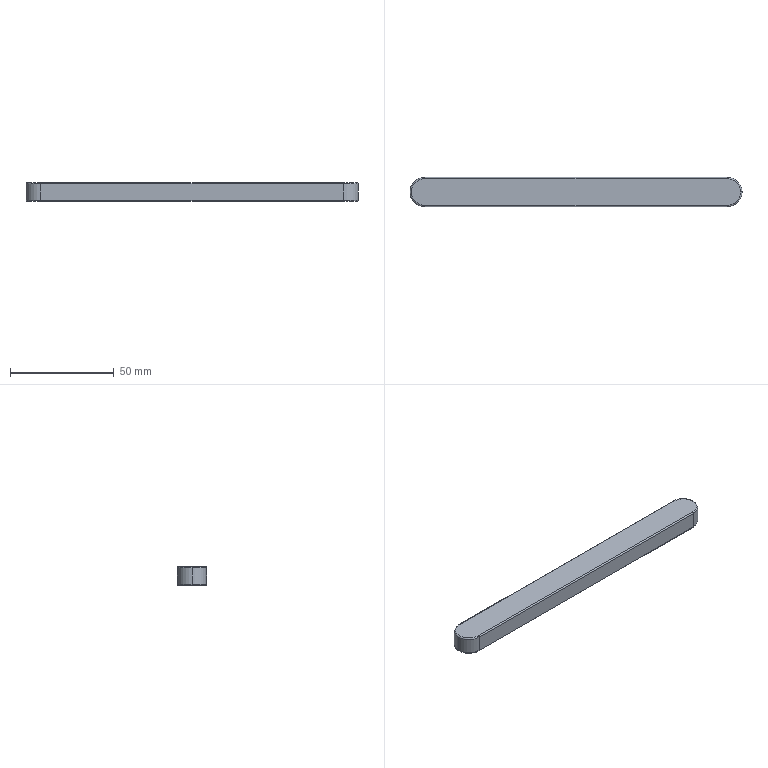Part | SolidWorks | features Extrusion 1, Fillet 1 | 1 solid | 17 faces | box 160 x 14 x 9 mm | volume 19730 mm3 | cylinder 7 | torus 6 | plane 4 | commonest cylinder face diameters 1.2 x4 14 x3
STEP:
#1=CARTESIAN_POINT('',(79.4,0.,0.));
#2=VERTEX_POINT('',#1);
#3=CARTESIAN_POINT('',(73.,-6.4,0.));
#4=VERTEX_POINT('',#3);
#5=CARTESIAN_POINT('',(73.,0.,0.));
#6=DIRECTION('',(0.,0.,-1.));
#7=DIRECTION('',(1.,0.,0.));
#8=AXIS2_PLACEMENT_3D('',#5,#6,#7);
#9=CIRCLE('',#8,6.4);
#10=EDGE_CURVE('',#2,#4,#9,.T.);
#11=ORIENTED_EDGE('',*,*,#10,.F.);
#12=CARTESIAN_POINT('',(80.,0.,0.6));
#13=VERTEX_POINT('',#12);
#14=CARTESIAN_POINT('',(79.4,0.,0.6));
#15=DIRECTION('',(0.,-1.,0.));
#16=DIRECTION('',(0.,0.,-1.));
#17=AXIS2_PLACEMENT_3D('',#14,#15,#16);
#18=CIRCLE('',#17,0.6);
#19=EDGE_CURVE('',#2,#13,#18,.T.);
#20=ORIENTED_EDGE('',*,*,#19,.T.);
#21=CARTESIAN_POINT('',(73.,-7.,0.6));
#22=VERTEX_POINT('',#21);
#23=CARTESIAN_POINT('',(73.,0.,0.6));
#24=DIRECTION('',(0.,0.,1.));
#25=DIRECTION('',(1.,0.,0.));
#26=AXIS2_PLACEMENT_3D('',#23,#24,#25);
#27=CIRCLE('',#26,7.);
#28=EDGE_CURVE('',#22,#13,#27,.T.);
#29=ORIENTED_EDGE('',*,*,#28,.F.);
#30=CARTESIAN_POINT('',(73.,-6.4,0.6));
#31=DIRECTION('',(1.,0.,0.));
#32=DIRECTION('',(0.,0.,-1.));
#33=AXIS2_PLACEMENT_3D('',#30,#31,#32);
#34=CIRCLE('',#33,0.6);
#35=EDGE_CURVE('',#22,#4,#34,.T.);
#36=ORIENTED_EDGE('',*,*,#35,.T.);
#37=EDGE_LOOP('',(#11,#20,#29,#36));
#38=FACE_OUTER_BOUND('',#37,.T.);
#39=CARTESIAN_POINT('',(73.,0.,0.6));
#40=DIRECTION('',(0.,0.,1.));
#41=DIRECTION('',(1.,0.,0.));
#42=AXIS2_PLACEMENT_3D('',#39,#40,#41);
#43=TOROIDAL_SURFACE('',#42,6.4,0.6);
#44=ADVANCED_FACE('',(#38),#43,.T.);
#45=CARTESIAN_POINT('',(80.,0.,8.4));
#46=VERTEX_POINT('',#45);
#47=CARTESIAN_POINT('',(73.,-7.,8.4));
#48=VERTEX_POINT('',#47);
#49=CARTESIAN_POINT('',(73.,0.,8.4));
#50=DIRECTION('',(0.,0.,-1.));
#51=DIRECTION('',(1.,0.,0.));
#52=AXIS2_PLACEMENT_3D('',#49,#50,#51);
#53=CIRCLE('',#52,7.);
#54=EDGE_CURVE('',#46,#48,#53,.T.);
#55=ORIENTED_EDGE('',*,*,#54,.F.);
#56=CARTESIAN_POINT('',(79.4,0.,9.));
#57=VERTEX_POINT('',#56);
#58=CARTESIAN_POINT('',(79.4,0.,8.4));
#59=DIRECTION('',(0.,-1.,0.));
#60=DIRECTION('',(0.,0.,-1.));
#61=AXIS2_PLACEMENT_3D('',#58,#59,#60);
#62=CIRCLE('',#61,0.6);
#63=EDGE_CURVE('',#46,#57,#62,.T.);
#64=ORIENTED_EDGE('',*,*,#63,.T.);
#65=CARTESIAN_POINT('',(73.,-6.4,9.));
#66=VERTEX_POINT('',#65);
#67=CARTESIAN_POINT('',(73.,0.,9.));
#68=DIRECTION('',(0.,0.,1.));
#69=DIRECTION('',(1.,0.,0.));
#70=AXIS2_PLACEMENT_3D('',#67,#68,#69);
#71=CIRCLE('',#70,6.4);
#72=EDGE_CURVE('',#66,#57,#71,.T.);
#73=ORIENTED_EDGE('',*,*,#72,.F.);
#74=CARTESIAN_POINT('',(73.,-6.4,8.4));
#75=DIRECTION('',(1.,0.,0.));
#76=DIRECTION('',(0.,0.,-1.));
#77=AXIS2_PLACEMENT_3D('',#74,#75,#76);
#78=CIRCLE('',#77,0.6);
#79=EDGE_CURVE('',#66,#48,#78,.T.);
#80=ORIENTED_EDGE('',*,*,#79,.T.);
#81=EDGE_LOOP('',(#55,#64,#73,#80));
#82=FACE_OUTER_BOUND('',#81,.T.);
#83=CARTESIAN_POINT('',(73.,0.,8.4));
#84=DIRECTION('',(0.,0.,1.));
#85=DIRECTION('',(1.,0.,0.));
#86=AXIS2_PLACEMENT_3D('',#83,#84,#85);
#87=TOROIDAL_SURFACE('',#86,6.4,0.6);
#88=ADVANCED_FACE('',(#82),#87,.T.);
#89=CARTESIAN_POINT('',(-73.,-7.,8.4));
#90=VERTEX_POINT('',#89);
#91=CARTESIAN_POINT('',(-80.,0.,8.4));
#92=VERTEX_POINT('',#91);
#93=CARTESIAN_POINT('',(-73.,0.,8.4));
#94=DIRECTION('',(0.,0.,-1.));
#95=DIRECTION('',(1.,0.,0.));
#96=AXIS2_PLACEMENT_3D('',#93,#94,#95);
#97=CIRCLE('',#96,7.);
#98=EDGE_CURVE('',#90,#92,#97,.T.);
#99=ORIENTED_EDGE('',*,*,#98,.T.);
#100=CARTESIAN_POINT('',(-80.,0.,0.6));
#101=VERTEX_POINT('',#100);
#102=CARTESIAN_POINT('',(-80.,0.,9.));
#103=DIRECTION('',(0.,0.,-1.));
#104=VECTOR('',#103,1000.);
#105=LINE('',#102,#104);
#106=EDGE_CURVE('',#92,#101,#105,.T.);
#107=ORIENTED_EDGE('',*,*,#106,.T.);
#108=CARTESIAN_POINT('',(-73.,-7.,0.6));
#109=VERTEX_POINT('',#108);
#110=CARTESIAN_POINT('',(-73.,0.,0.6));
#111=DIRECTION('',(0.,0.,1.));
#112=DIRECTION('',(1.,0.,0.));
#113=AXIS2_PLACEMENT_3D('',#110,#111,#112);
#114=CIRCLE('',#113,7.);
#115=EDGE_CURVE('',#101,#109,#114,.T.);
#116=ORIENTED_EDGE('',*,*,#115,.T.);
#117=CARTESIAN_POINT('',(-73.,-7.,9.));
#118=DIRECTION('',(0.,0.,-1.));
#119=VECTOR('',#118,1000.);
#120=LINE('',#117,#119);
#121=EDGE_CURVE('',#90,#109,#120,.T.);
#122=ORIENTED_EDGE('',*,*,#121,.F.);
#123=EDGE_LOOP('',(#99,#107,#116,#122));
#124=FACE_OUTER_BOUND('',#123,.T.);
#125=CARTESIAN_POINT('',(-73.,0.,9.));
#126=DIRECTION('',(0.,0.,-1.));
#127=DIRECTION('',(-1.,0.,0.));
#128=AXIS2_PLACEMENT_3D('',#125,#126,#127);
#129=CYLINDRICAL_SURFACE('',#128,7.);
#130=ADVANCED_FACE('',(#124),#129,.T.);
#131=ORIENTED_EDGE('',*,*,#106,.F.);
#132=CARTESIAN_POINT('',(-73.,7.,8.4));
#133=VERTEX_POINT('',#132);
#134=CARTESIAN_POINT('',(-73.,0.,8.4));
#135=DIRECTION('',(0.,0.,-1.));
#136=DIRECTION('',(1.,0.,0.));
#137=AXIS2_PLACEMENT_3D('',#134,#135,#136);
#138=CIRCLE('',#137,7.);
#139=EDGE_CURVE('',#92,#133,#138,.T.);
#140=ORIENTED_EDGE('',*,*,#139,.T.);
#141=CARTESIAN_POINT('',(-73.,7.,0.6));
#142=VERTEX_POINT('',#141);
#143=CARTESIAN_POINT('',(-73.,7.,9.));
#144=DIRECTION('',(0.,0.,-1.));
#145=VECTOR('',#144,1000.);
#146=LINE('',#143,#145);
#147=EDGE_CURVE('',#133,#142,#146,.T.);
#148=ORIENTED_EDGE('',*,*,#147,.T.);
#149=CARTESIAN_POINT('',(-73.,0.,0.6));
#150=DIRECTION('',(0.,0.,1.));
#151=DIRECTION('',(1.,0.,0.));
#152=AXIS2_PLACEMENT_3D('',#149,#150,#151);
#153=CIRCLE('',#152,7.);
#154=EDGE_CURVE('',#142,#101,#153,.T.);
#155=ORIENTED_EDGE('',*,*,#154,.T.);
#156=EDGE_LOOP('',(#131,#140,#148,#155));
#157=FACE_OUTER_BOUND('',#156,.T.);
#158=CARTESIAN_POINT('',(-73.,0.,9.));
#159=DIRECTION('',(0.,0.,-1.));
#160=DIRECTION('',(-1.,0.,0.));
#161=AXIS2_PLACEMENT_3D('',#158,#159,#160);
#162=CYLINDRICAL_SURFACE('',#161,7.);
#163=ADVANCED_FACE('',(#157),#162,.T.);
#164=CARTESIAN_POINT('',(73.,-7.,9.));
#165=DIRECTION('',(0.,0.,-1.));
#166=VECTOR('',#165,1000.);
#167=LINE('',#164,#166);
#168=EDGE_CURVE('',#48,#22,#167,.T.);
#169=ORIENTED_EDGE('',*,*,#168,.F.);
#170=CARTESIAN_POINT('',(-73.,-7.,8.4));
#171=DIRECTION('',(-1.,0.,0.));
#172=VECTOR('',#171,1000.);
#173=LINE('',#170,#172);
#174=EDGE_CURVE('',#48,#90,#173,.T.);
#175=ORIENTED_EDGE('',*,*,#174,.T.);
#176=ORIENTED_EDGE('',*,*,#121,.T.);
#177=CARTESIAN_POINT('',(-73.,-7.,0.6));
#178=DIRECTION('',(1.,0.,0.));
#179=VECTOR('',#178,1000.);
#180=LINE('',#177,#179);
#181=EDGE_CURVE('',#109,#22,#180,.T.);
#182=ORIENTED_EDGE('',*,*,#181,.T.);
#183=EDGE_LOOP('',(#169,#175,#176,#182));
#184=FACE_OUTER_BOUND('',#183,.T.);
#185=CARTESIAN_POINT('',(-73.,-7.,9.));
#186=DIRECTION('',(0.,1.,0.));
#187=DIRECTION('',(-1.,0.,0.));
#188=AXIS2_PLACEMENT_3D('',#185,#186,#187);
#189=PLANE('',#188);
#190=ADVANCED_FACE('',(#184),#189,.F.);
#191=CARTESIAN_POINT('',(73.,7.,8.4));
#192=VERTEX_POINT('',#191);
#193=CARTESIAN_POINT('',(73.,7.,0.6));
#194=VERTEX_POINT('',#193);
#195=CARTESIAN_POINT('',(73.,7.,9.));
#196=DIRECTION('',(0.,0.,-1.));
#197=VECTOR('',#196,1000.);
#198=LINE('',#195,#197);
#199=EDGE_CURVE('',#192,#194,#198,.T.);
#200=ORIENTED_EDGE('',*,*,#199,.F.);
#201=CARTESIAN_POINT('',(73.,0.,8.4));
#202=DIRECTION('',(0.,0.,-1.));
#203=DIRECTION('',(1.,0.,0.));
#204=AXIS2_PLACEMENT_3D('',#201,#202,#203);
#205=CIRCLE('',#204,7.);
#206=EDGE_CURVE('',#192,#46,#205,.T.);
#207=ORIENTED_EDGE('',*,*,#206,.T.);
#208=ORIENTED_EDGE('',*,*,#54,.T.);
#209=ORIENTED_EDGE('',*,*,#168,.T.);
#210=ORIENTED_EDGE('',*,*,#28,.T.);
#211=CARTESIAN_POINT('',(73.,0.,0.6));
#212=DIRECTION('',(0.,0.,1.));
#213=DIRECTION('',(1.,0.,0.));
#214=AXIS2_PLACEMENT_3D('',#211,#212,#213);
#215=CIRCLE('',#214,7.);
#216=EDGE_CURVE('',#13,#194,#215,.T.);
#217=ORIENTED_EDGE('',*,*,#216,.T.);
#218=EDGE_LOOP('',(#200,#207,#208,#209,#210,#217));
#219=FACE_OUTER_BOUND('',#218,.T.);
#220=CARTESIAN_POINT('',(73.,0.,9.));
#221=DIRECTION('',(0.,0.,-1.));
#222=DIRECTION('',(-1.,0.,0.));
#223=AXIS2_PLACEMENT_3D('',#220,#221,#222);
#224=CYLINDRICAL_SURFACE('',#223,7.);
#225=ADVANCED_FACE('',(#219),#224,.T.);
#226=ORIENTED_EDGE('',*,*,#147,.F.);
#227=CARTESIAN_POINT('',(73.,7.,8.4));
#228=DIRECTION('',(1.,0.,0.));
#229=VECTOR('',#228,1000.);
#230=LINE('',#227,#229);
#231=EDGE_CURVE('',#133,#192,#230,.T.);
#232=ORIENTED_EDGE('',*,*,#231,.T.);
#233=ORIENTED_EDGE('',*,*,#199,.T.);
#234=CARTESIAN_POINT('',(-73.,7.,0.6));
#235=DIRECTION('',(-1.,0.,0.));
#236=VECTOR('',#235,1000.);
#237=LINE('',#234,#236);
#238=EDGE_CURVE('',#194,#142,#237,.T.);
#239=ORIENTED_EDGE('',*,*,#238,.T.);
#240=EDGE_LOOP('',(#226,#232,#233,#239));
#241=FACE_OUTER_BOUND('',#240,.T.);
#242=CARTESIAN_POINT('',(-73.,7.,9.));
#243=DIRECTION('',(0.,-1.,0.));
#244=DIRECTION('',(1.,0.,0.));
#245=AXIS2_PLACEMENT_3D('',#242,#243,#244);
#246=PLANE('',#245);
#247=ADVANCED_FACE('',(#241),#246,.F.);
#248=CARTESIAN_POINT('',(-73.,-6.4,9.));
#249=VERTEX_POINT('',#248);
#250=CARTESIAN_POINT('',(73.,-6.4,9.));
#251=DIRECTION('',(1.,0.,0.));
#252=VECTOR('',#251,1000.);
#253=LINE('',#250,#252);
#254=EDGE_CURVE('',#249,#66,#253,.T.);
#255=ORIENTED_EDGE('',*,*,#254,.T.);
#256=ORIENTED_EDGE('',*,*,#72,.T.);
#257=CARTESIAN_POINT('',(73.,6.4,9.));
#258=VERTEX_POINT('',#257);
#259=CARTESIAN_POINT('',(73.,0.,9.));
#260=DIRECTION('',(0.,0.,1.));
#261=DIRECTION('',(1.,0.,0.));
#262=AXIS2_PLACEMENT_3D('',#259,#260,#261);
#263=CIRCLE('',#262,6.4);
#264=EDGE_CURVE('',#57,#258,#263,.T.);
#265=ORIENTED_EDGE('',*,*,#264,.T.);
#266=CARTESIAN_POINT('',(-73.,6.4,9.));
#267=VERTEX_POINT('',#266);
#268=CARTESIAN_POINT('',(-73.,6.4,9.));
#269=DIRECTION('',(-1.,0.,0.));
#270=VECTOR('',#269,1000.);
#271=LINE('',#268,#270);
#272=EDGE_CURVE('',#258,#267,#271,.T.);
#273=ORIENTED_EDGE('',*,*,#272,.T.);
#274=CARTESIAN_POINT('',(-73.,0.,9.));
#275=DIRECTION('',(0.,0.,1.));
#276=DIRECTION('',(1.,0.,0.));
#277=AXIS2_PLACEMENT_3D('',#274,#275,#276);
#278=CIRCLE('',#277,6.4);
#279=EDGE_CURVE('',#267,#249,#278,.T.);
#280=ORIENTED_EDGE('',*,*,#279,.T.);
#281=EDGE_LOOP('',(#255,#256,#265,#273,#280));
#282=FACE_OUTER_BOUND('',#281,.T.);
#283=CARTESIAN_POINT('',(-73.,0.,9.));
#284=DIRECTION('',(0.,0.,1.));
#285=DIRECTION('',(1.,0.,0.));
#286=AXIS2_PLACEMENT_3D('',#283,#284,#285);
#287=PLANE('',#286);
#288=ADVANCED_FACE('',(#282),#287,.T.);
#289=CARTESIAN_POINT('',(-73.,6.4,0.));
#290=VERTEX_POINT('',#289);
#291=CARTESIAN_POINT('',(73.,6.4,0.));
#292=VERTEX_POINT('',#291);
#293=CARTESIAN_POINT('',(-73.,6.4,0.));
#294=DIRECTION('',(1.,0.,0.));
#295=VECTOR('',#294,1000.);
#296=LINE('',#293,#295);
#297=EDGE_CURVE('',#290,#292,#296,.T.);
#298=ORIENTED_EDGE('',*,*,#297,.T.);
#299=CARTESIAN_POINT('',(73.,0.,0.));
#300=DIRECTION('',(0.,0.,-1.));
#301=DIRECTION('',(1.,0.,0.));
#302=AXIS2_PLACEMENT_3D('',#299,#300,#301);
#303=CIRCLE('',#302,6.4);
#304=EDGE_CURVE('',#292,#2,#303,.T.);
#305=ORIENTED_EDGE('',*,*,#304,.T.);
#306=ORIENTED_EDGE('',*,*,#10,.T.);
#307=CARTESIAN_POINT('',(-73.,-6.4,0.));
#308=VERTEX_POINT('',#307);
#309=CARTESIAN_POINT('',(-73.,-6.4,0.));
#310=DIRECTION('',(-1.,0.,0.));
#311=VECTOR('',#310,1000.);
#312=LINE('',#309,#311);
#313=EDGE_CURVE('',#4,#308,#312,.T.);
#314=ORIENTED_EDGE('',*,*,#313,.T.);
#315=CARTESIAN_POINT('',(-73.,0.,0.));
#316=DIRECTION('',(0.,0.,-1.));
#317=DIRECTION('',(1.,0.,0.));
#318=AXIS2_PLACEMENT_3D('',#315,#316,#317);
#319=CIRCLE('',#318,6.4);
#320=EDGE_CURVE('',#308,#290,#319,.T.);
#321=ORIENTED_EDGE('',*,*,#320,.T.);
#322=EDGE_LOOP('',(#298,#305,#306,#314,#321));
#323=FACE_OUTER_BOUND('',#322,.T.);
#324=CARTESIAN_POINT('',(-73.,0.,0.));
#325=DIRECTION('',(0.,0.,1.));
#326=DIRECTION('',(1.,0.,0.));
#327=AXIS2_PLACEMENT_3D('',#324,#325,#326);
#328=PLANE('',#327);
#329=ADVANCED_FACE('',(#323),#328,.F.);
#330=CARTESIAN_POINT('',(-73.,6.4,8.4));
#331=DIRECTION('',(1.,0.,0.));
#332=DIRECTION('',(0.,0.,-1.));
#333=AXIS2_PLACEMENT_3D('',#330,#331,#332);
#334=CIRCLE('',#333,0.6);
#335=EDGE_CURVE('',#133,#267,#334,.T.);
#336=ORIENTED_EDGE('',*,*,#335,.F.);
#337=ORIENTED_EDGE('',*,*,#139,.F.);
#338=ORIENTED_EDGE('',*,*,#98,.F.);
#339=CARTESIAN_POINT('',(-73.,-6.4,8.4));
#340=DIRECTION('',(1.,0.,0.));
#341=DIRECTION('',(0.,0.,-1.));
#342=AXIS2_PLACEMENT_3D('',#339,#340,#341);
#343=CIRCLE('',#342,0.6);
#344=EDGE_CURVE('',#249,#90,#343,.T.);
#345=ORIENTED_EDGE('',*,*,#344,.F.);
#346=ORIENTED_EDGE('',*,*,#279,.F.);
#347=EDGE_LOOP('',(#336,#337,#338,#345,#346));
#348=FACE_OUTER_BOUND('',#347,.T.);
#349=CARTESIAN_POINT('',(-73.,0.,8.4));
#350=DIRECTION('',(0.,0.,1.));
#351=DIRECTION('',(1.,0.,0.));
#352=AXIS2_PLACEMENT_3D('',#349,#350,#351);
#353=TOROIDAL_SURFACE('',#352,6.4,0.6);
#354=ADVANCED_FACE('',(#348),#353,.T.);
#355=ORIENTED_EDGE('',*,*,#344,.T.);
#356=ORIENTED_EDGE('',*,*,#174,.F.);
#357=ORIENTED_EDGE('',*,*,#79,.F.);
#358=ORIENTED_EDGE('',*,*,#254,.F.);
#359=EDGE_LOOP('',(#355,#356,#357,#358));
#360=FACE_OUTER_BOUND('',#359,.T.);
#361=CARTESIAN_POINT('',(-73.,-6.4,8.4));
#362=DIRECTION('',(-1.,0.,0.));
#363=DIRECTION('',(0.,-1.,0.));
#364=AXIS2_PLACEMENT_3D('',#361,#362,#363);
#365=CYLINDRICAL_SURFACE('',#364,0.6);
#366=ADVANCED_FACE('',(#360),#365,.T.);
#367=ORIENTED_EDGE('',*,*,#335,.T.);
#368=ORIENTED_EDGE('',*,*,#272,.F.);
#369=CARTESIAN_POINT('',(73.,6.4,8.4));
#370=DIRECTION('',(1.,0.,0.));
#371=DIRECTION('',(0.,0.,-1.));
#372=AXIS2_PLACEMENT_3D('',#369,#370,#371);
#373=CIRCLE('',#372,0.6);
#374=EDGE_CURVE('',#192,#258,#373,.T.);
#375=ORIENTED_EDGE('',*,*,#374,.F.);
#376=ORIENTED_EDGE('',*,*,#231,.F.);
#377=EDGE_LOOP('',(#367,#368,#375,#376));
#378=FACE_OUTER_BOUND('',#377,.T.);
#379=CARTESIAN_POINT('',(-73.,6.4,8.4));
#380=DIRECTION('',(1.,0.,0.));
#381=DIRECTION('',(0.,1.,0.));
#382=AXIS2_PLACEMENT_3D('',#379,#380,#381);
#383=CYLINDRICAL_SURFACE('',#382,0.6);
#384=ADVANCED_FACE('',(#378),#383,.T.);
#385=ORIENTED_EDGE('',*,*,#63,.F.);
#386=ORIENTED_EDGE('',*,*,#206,.F.);
#387=ORIENTED_EDGE('',*,*,#374,.T.);
#388=ORIENTED_EDGE('',*,*,#264,.F.);
#389=EDGE_LOOP('',(#385,#386,#387,#388));
#390=FACE_OUTER_BOUND('',#389,.T.);
#391=CARTESIAN_POINT('',(73.,0.,8.4));
#392=DIRECTION('',(0.,0.,1.));
#393=DIRECTION('',(1.,0.,0.));
#394=AXIS2_PLACEMENT_3D('',#391,#392,#393);
#395=TOROIDAL_SURFACE('',#394,6.4,0.6);
#396=ADVANCED_FACE('',(#390),#395,.T.);
#397=CARTESIAN_POINT('',(-73.,6.4,0.6));
#398=DIRECTION('',(1.,0.,0.));
#399=DIRECTION('',(0.,0.,-1.));
#400=AXIS2_PLACEMENT_3D('',#397,#398,#399);
#401=CIRCLE('',#400,0.6);
#402=EDGE_CURVE('',#290,#142,#401,.T.);
#403=ORIENTED_EDGE('',*,*,#402,.F.);
#404=ORIENTED_EDGE('',*,*,#320,.F.);
#405=CARTESIAN_POINT('',(-73.,-6.4,0.6));
#406=DIRECTION('',(1.,0.,0.));
#407=DIRECTION('',(0.,0.,-1.));
#408=AXIS2_PLACEMENT_3D('',#405,#406,#407);
#409=CIRCLE('',#408,0.6);
#410=EDGE_CURVE('',#109,#308,#409,.T.);
#411=ORIENTED_EDGE('',*,*,#410,.F.);
#412=ORIENTED_EDGE('',*,*,#115,.F.);
#413=ORIENTED_EDGE('',*,*,#154,.F.);
#414=EDGE_LOOP('',(#403,#404,#411,#412,#413));
#415=FACE_OUTER_BOUND('',#414,.T.);
#416=CARTESIAN_POINT('',(-73.,0.,0.6));
#417=DIRECTION('',(0.,0.,1.));
#418=DIRECTION('',(1.,0.,0.));
#419=AXIS2_PLACEMENT_3D('',#416,#417,#418);
#420=TOROIDAL_SURFACE('',#419,6.4,0.6);
#421=ADVANCED_FACE('',(#415),#420,.T.);
#422=ORIENTED_EDGE('',*,*,#410,.T.);
#423=ORIENTED_EDGE('',*,*,#313,.F.);
#424=ORIENTED_EDGE('',*,*,#35,.F.);
#425=ORIENTED_EDGE('',*,*,#181,.F.);
#426=EDGE_LOOP('',(#422,#423,#424,#425));
#427=FACE_OUTER_BOUND('',#426,.T.);
#428=CARTESIAN_POINT('',(-73.,-6.4,0.6));
#429=DIRECTION('',(1.,0.,0.));
#430=DIRECTION('',(0.,1.,0.));
#431=AXIS2_PLACEMENT_3D('',#428,#429,#430);
#432=CYLINDRICAL_SURFACE('',#431,0.6);
#433=ADVANCED_FACE('',(#427),#432,.T.);
#434=ORIENTED_EDGE('',*,*,#402,.T.);
#435=ORIENTED_EDGE('',*,*,#238,.F.);
#436=CARTESIAN_POINT('',(73.,6.4,0.6));
#437=DIRECTION('',(1.,0.,0.));
#438=DIRECTION('',(0.,0.,-1.));
#439=AXIS2_PLACEMENT_3D('',#436,#437,#438);
#440=CIRCLE('',#439,0.6);
#441=EDGE_CURVE('',#292,#194,#440,.T.);
#442=ORIENTED_EDGE('',*,*,#441,.F.);
#443=ORIENTED_EDGE('',*,*,#297,.F.);
#444=EDGE_LOOP('',(#434,#435,#442,#443));
#445=FACE_OUTER_BOUND('',#444,.T.);
#446=CARTESIAN_POINT('',(-73.,6.4,0.6));
#447=DIRECTION('',(-1.,0.,0.));
#448=DIRECTION('',(0.,-1.,0.));
#449=AXIS2_PLACEMENT_3D('',#446,#447,#448);
#450=CYLINDRICAL_SURFACE('',#449,0.6);
#451=ADVANCED_FACE('',(#445),#450,.T.);
#452=ORIENTED_EDGE('',*,*,#19,.F.);
#453=ORIENTED_EDGE('',*,*,#304,.F.);
#454=ORIENTED_EDGE('',*,*,#441,.T.);
#455=ORIENTED_EDGE('',*,*,#216,.F.);
#456=EDGE_LOOP('',(#452,#453,#454,#455));
#457=FACE_OUTER_BOUND('',#456,.T.);
#458=CARTESIAN_POINT('',(73.,0.,0.6));
#459=DIRECTION('',(0.,0.,1.));
#460=DIRECTION('',(1.,0.,0.));
#461=AXIS2_PLACEMENT_3D('',#458,#459,#460);
#462=TOROIDAL_SURFACE('',#461,6.4,0.6);
#463=ADVANCED_FACE('',(#457),#462,.T.);
#464=CLOSED_SHELL('',(#44,#88,#130,#163,#190,#225,#247,#288,#329,#354,#366,#384,#396,#421,#433,#451,#463));
#465=MANIFOLD_SOLID_BREP('',#464);
#466=CARTESIAN_POINT('',(0.,0.,0.));
#467=DIRECTION('',(0.,0.,1.));
#468=DIRECTION('',(1.,0.,0.));
#469=AXIS2_PLACEMENT_3D('',#466,#467,#468);
#470=(LENGTH_UNIT()NAMED_UNIT(*)SI_UNIT(.MILLI.,.METRE.));
#471=UNCERTAINTY_MEASURE_WITH_UNIT(LENGTH_MEASURE(0.00001),#470,'','');
#472=(NAMED_UNIT(*)PLANE_ANGLE_UNIT()SI_UNIT($,.RADIAN.));
#473=(NAMED_UNIT(*)SI_UNIT($,.STERADIAN.)SOLID_ANGLE_UNIT());
#474=(GEOMETRIC_REPRESENTATION_CONTEXT(3)GLOBAL_UNCERTAINTY_ASSIGNED_CONTEXT((#471))GLOBAL_UNIT_ASSIGNED_CONTEXT((#470,#472,#473))REPRESENTATION_CONTEXT('',''));
#475=ADVANCED_BREP_SHAPE_REPRESENTATION('',(#465,#469),#474);